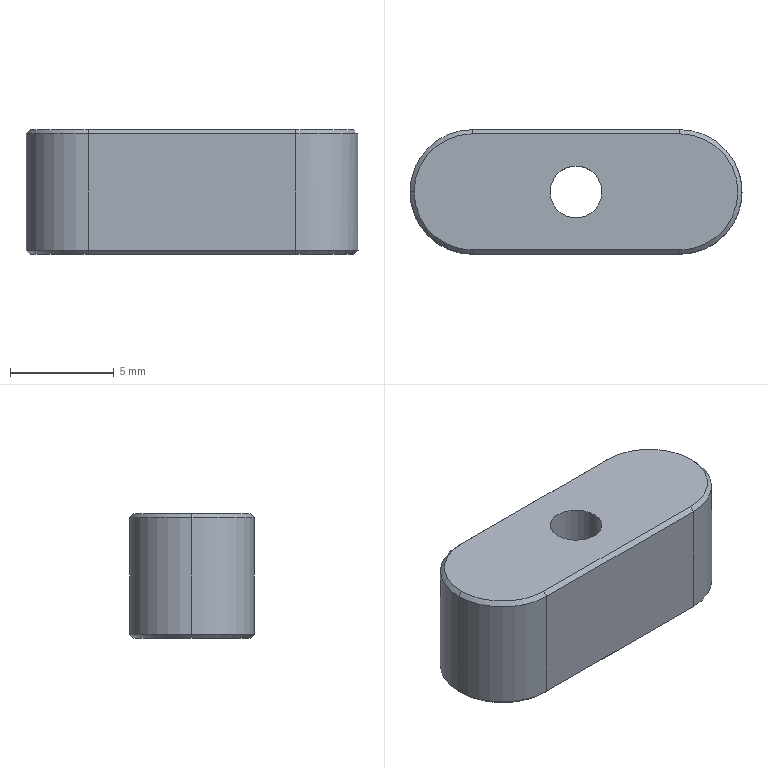Part | NX | features BREP 1 | 1 solid | 19 faces | box 16 x 6 x 6 mm | volume 498.656 mm3 | plane 8 | cone 6 | cylinder 5 | commonest cylinder face diameters 6 x3 2.5 x2
STEP:
#1=CARTESIAN_POINT('',(1.25,0.,-3.));
#2=VERTEX_POINT('',#1);
#3=CARTESIAN_POINT('',(-1.25,0.,-3.));
#4=VERTEX_POINT('',#3);
#5=CARTESIAN_POINT('',(0.,0.,-3.));
#6=DIRECTION('',(0.,0.,-1.));
#7=DIRECTION('',(-1.,0.,0.));
#8=AXIS2_PLACEMENT_3D('',#5,#6,#7);
#9=CIRCLE('',#8,1.25);
#10=EDGE_CURVE('',#2,#4,#9,.T.);
#11=ORIENTED_EDGE('',*,*,#10,.T.);
#12=CARTESIAN_POINT('',(-1.25,0.,3.));
#13=VERTEX_POINT('',#12);
#14=CARTESIAN_POINT('',(-1.25,0.,3.));
#15=DIRECTION('',(0.,0.,1.));
#16=VECTOR('',#15,1000.);
#17=LINE('',#14,#16);
#18=EDGE_CURVE('',#13,#4,#17,.F.);
#19=ORIENTED_EDGE('',*,*,#18,.F.);
#20=CARTESIAN_POINT('',(1.25,0.,3.));
#21=VERTEX_POINT('',#20);
#22=CARTESIAN_POINT('',(0.,0.,3.));
#23=DIRECTION('',(0.,0.,1.));
#24=DIRECTION('',(1.,0.,0.));
#25=AXIS2_PLACEMENT_3D('',#22,#23,#24);
#26=CIRCLE('',#25,1.25);
#27=EDGE_CURVE('',#13,#21,#26,.T.);
#28=ORIENTED_EDGE('',*,*,#27,.T.);
#29=CARTESIAN_POINT('',(1.25,0.,3.));
#30=DIRECTION('',(0.,0.,1.));
#31=VECTOR('',#30,1000.);
#32=LINE('',#29,#31);
#33=EDGE_CURVE('',#21,#2,#32,.F.);
#34=ORIENTED_EDGE('',*,*,#33,.T.);
#35=EDGE_LOOP('',(#11,#19,#28,#34));
#36=FACE_BOUND('',#35,.T.);
#37=CARTESIAN_POINT('',(0.,0.,3.));
#38=DIRECTION('',(0.,0.,1.));
#39=DIRECTION('',(1.,0.,0.));
#40=AXIS2_PLACEMENT_3D('',#37,#38,#39);
#41=CYLINDRICAL_SURFACE('',#40,1.25);
#42=ADVANCED_FACE('',(#36),#41,.F.);
#43=CARTESIAN_POINT('',(-7.8,0.,3.));
#44=VERTEX_POINT('',#43);
#45=CARTESIAN_POINT('',(-5.,-2.8,3.));
#46=VERTEX_POINT('',#45);
#47=CARTESIAN_POINT('',(-5.,0.,3.));
#48=DIRECTION('',(0.,0.,1.));
#49=DIRECTION('',(-1.,0.,0.));
#50=AXIS2_PLACEMENT_3D('',#47,#48,#49);
#51=CIRCLE('',#50,2.8);
#52=EDGE_CURVE('',#44,#46,#51,.T.);
#53=ORIENTED_EDGE('',*,*,#52,.F.);
#54=CARTESIAN_POINT('',(-8.,0.,2.8));
#55=VERTEX_POINT('',#54);
#56=CARTESIAN_POINT('',(-7.8,0.,3.));
#57=DIRECTION('',(-0.7071,0.,-0.7071));
#58=VECTOR('',#57,1000.);
#59=LINE('',#56,#58);
#60=EDGE_CURVE('',#44,#55,#59,.T.);
#61=ORIENTED_EDGE('',*,*,#60,.T.);
#62=CARTESIAN_POINT('',(-5.,-3.,2.8));
#63=VERTEX_POINT('',#62);
#64=CARTESIAN_POINT('',(-5.,0.,2.8));
#65=DIRECTION('',(0.,0.,-1.));
#66=DIRECTION('',(-1.,0.,0.));
#67=AXIS2_PLACEMENT_3D('',#64,#65,#66);
#68=CIRCLE('',#67,3.);
#69=EDGE_CURVE('',#63,#55,#68,.T.);
#70=ORIENTED_EDGE('',*,*,#69,.F.);
#71=CARTESIAN_POINT('',(-5.,-2.8,3.));
#72=DIRECTION('',(0.,-0.7071,-0.7071));
#73=VECTOR('',#72,1000.);
#74=LINE('',#71,#73);
#75=EDGE_CURVE('',#46,#63,#74,.T.);
#76=ORIENTED_EDGE('',*,*,#75,.F.);
#77=EDGE_LOOP('',(#53,#61,#70,#76));
#78=FACE_BOUND('',#77,.T.);
#79=CARTESIAN_POINT('',(-5.,0.,3.));
#80=DIRECTION('',(0.,0.,-1.));
#81=DIRECTION('',(-1.,0.,0.));
#82=AXIS2_PLACEMENT_3D('',#79,#80,#81);
#83=CONICAL_SURFACE('',#82,2.8,0.7854);
#84=ADVANCED_FACE('',(#78),#83,.T.);
#85=CARTESIAN_POINT('',(7.8,0.,-3.));
#86=VERTEX_POINT('',#85);
#87=CARTESIAN_POINT('',(5.,-2.8,-3.));
#88=VERTEX_POINT('',#87);
#89=CARTESIAN_POINT('',(5.,0.,-3.));
#90=DIRECTION('',(0.,0.,-1.));
#91=DIRECTION('',(-1.,0.,0.));
#92=AXIS2_PLACEMENT_3D('',#89,#90,#91);
#93=CIRCLE('',#92,2.8);
#94=EDGE_CURVE('',#86,#88,#93,.T.);
#95=ORIENTED_EDGE('',*,*,#94,.F.);
#96=CARTESIAN_POINT('',(8.,0.,-2.8));
#97=VERTEX_POINT('',#96);
#98=CARTESIAN_POINT('',(8.,0.,-2.8));
#99=DIRECTION('',(0.7071,0.,0.7071));
#100=VECTOR('',#99,1000.);
#101=LINE('',#98,#100);
#102=EDGE_CURVE('',#86,#97,#101,.T.);
#103=ORIENTED_EDGE('',*,*,#102,.T.);
#104=CARTESIAN_POINT('',(5.,-3.,-2.8));
#105=VERTEX_POINT('',#104);
#106=CARTESIAN_POINT('',(5.,0.,-2.8));
#107=DIRECTION('',(0.,0.,1.));
#108=DIRECTION('',(-1.,0.,0.));
#109=AXIS2_PLACEMENT_3D('',#106,#107,#108);
#110=CIRCLE('',#109,3.);
#111=EDGE_CURVE('',#105,#97,#110,.T.);
#112=ORIENTED_EDGE('',*,*,#111,.F.);
#113=CARTESIAN_POINT('',(5.,-3.,-2.8));
#114=DIRECTION('',(0.,0.7071,-0.7071));
#115=VECTOR('',#114,1000.);
#116=LINE('',#113,#115);
#117=EDGE_CURVE('',#105,#88,#116,.T.);
#118=ORIENTED_EDGE('',*,*,#117,.T.);
#119=EDGE_LOOP('',(#95,#103,#112,#118));
#120=FACE_BOUND('',#119,.T.);
#121=CARTESIAN_POINT('',(5.,0.,-2.8));
#122=DIRECTION('',(0.,0.,1.));
#123=DIRECTION('',(1.,0.,0.));
#124=AXIS2_PLACEMENT_3D('',#121,#122,#123);
#125=CONICAL_SURFACE('',#124,3.,0.7854);
#126=ADVANCED_FACE('',(#120),#125,.T.);
#127=ORIENTED_EDGE('',*,*,#69,.T.);
#128=CARTESIAN_POINT('',(-8.,0.,-2.8));
#129=VERTEX_POINT('',#128);
#130=CARTESIAN_POINT('',(-8.,0.,3.));
#131=DIRECTION('',(0.,0.,-1.));
#132=VECTOR('',#131,1000.);
#133=LINE('',#130,#132);
#134=EDGE_CURVE('',#55,#129,#133,.T.);
#135=ORIENTED_EDGE('',*,*,#134,.T.);
#136=CARTESIAN_POINT('',(-5.,-3.,-2.8));
#137=VERTEX_POINT('',#136);
#138=CARTESIAN_POINT('',(-5.,0.,-2.8));
#139=DIRECTION('',(0.,0.,1.));
#140=DIRECTION('',(-1.,0.,0.));
#141=AXIS2_PLACEMENT_3D('',#138,#139,#140);
#142=CIRCLE('',#141,3.);
#143=EDGE_CURVE('',#129,#137,#142,.T.);
#144=ORIENTED_EDGE('',*,*,#143,.T.);
#145=CARTESIAN_POINT('',(-5.,-3.,3.));
#146=DIRECTION('',(0.,0.,-1.));
#147=VECTOR('',#146,1000.);
#148=LINE('',#145,#147);
#149=EDGE_CURVE('',#63,#137,#148,.T.);
#150=ORIENTED_EDGE('',*,*,#149,.F.);
#151=EDGE_LOOP('',(#127,#135,#144,#150));
#152=FACE_BOUND('',#151,.T.);
#153=CARTESIAN_POINT('',(-5.,0.,3.));
#154=DIRECTION('',(0.,0.,-1.));
#155=DIRECTION('',(-1.,0.,0.));
#156=AXIS2_PLACEMENT_3D('',#153,#154,#155);
#157=CYLINDRICAL_SURFACE('',#156,3.);
#158=ADVANCED_FACE('',(#152),#157,.T.);
#159=CARTESIAN_POINT('',(5.,-3.,2.8));
#160=VERTEX_POINT('',#159);
#161=CARTESIAN_POINT('',(5.,-3.,3.));
#162=DIRECTION('',(0.,0.,-1.));
#163=VECTOR('',#162,1000.);
#164=LINE('',#161,#163);
#165=EDGE_CURVE('',#160,#105,#164,.T.);
#166=ORIENTED_EDGE('',*,*,#165,.T.);
#167=ORIENTED_EDGE('',*,*,#111,.T.);
#168=CARTESIAN_POINT('',(5.,3.,-2.8));
#169=VERTEX_POINT('',#168);
#170=CARTESIAN_POINT('',(5.,0.,-2.8));
#171=DIRECTION('',(0.,0.,1.));
#172=DIRECTION('',(-1.,0.,0.));
#173=AXIS2_PLACEMENT_3D('',#170,#171,#172);
#174=CIRCLE('',#173,3.);
#175=EDGE_CURVE('',#97,#169,#174,.T.);
#176=ORIENTED_EDGE('',*,*,#175,.T.);
#177=CARTESIAN_POINT('',(5.,3.,2.8));
#178=VERTEX_POINT('',#177);
#179=CARTESIAN_POINT('',(5.,3.,3.));
#180=DIRECTION('',(0.,0.,-1.));
#181=VECTOR('',#180,1000.);
#182=LINE('',#179,#181);
#183=EDGE_CURVE('',#178,#169,#182,.T.);
#184=ORIENTED_EDGE('',*,*,#183,.F.);
#185=CARTESIAN_POINT('',(5.,0.,2.8));
#186=DIRECTION('',(0.,0.,-1.));
#187=DIRECTION('',(-1.,0.,0.));
#188=AXIS2_PLACEMENT_3D('',#185,#186,#187);
#189=CIRCLE('',#188,3.);
#190=EDGE_CURVE('',#178,#160,#189,.T.);
#191=ORIENTED_EDGE('',*,*,#190,.T.);
#192=EDGE_LOOP('',(#166,#167,#176,#184,#191));
#193=FACE_BOUND('',#192,.T.);
#194=CARTESIAN_POINT('',(5.,0.,3.));
#195=DIRECTION('',(0.,0.,-1.));
#196=DIRECTION('',(-1.,0.,0.));
#197=AXIS2_PLACEMENT_3D('',#194,#195,#196);
#198=CYLINDRICAL_SURFACE('',#197,3.);
#199=ADVANCED_FACE('',(#193),#198,.T.);
#200=ORIENTED_EDGE('',*,*,#183,.T.);
#201=CARTESIAN_POINT('',(-5.,3.,-2.8));
#202=VERTEX_POINT('',#201);
#203=CARTESIAN_POINT('',(-5.,3.,-2.8));
#204=DIRECTION('',(-1.,0.,0.));
#205=VECTOR('',#204,1000.);
#206=LINE('',#203,#205);
#207=EDGE_CURVE('',#169,#202,#206,.T.);
#208=ORIENTED_EDGE('',*,*,#207,.T.);
#209=CARTESIAN_POINT('',(-5.,3.,2.8));
#210=VERTEX_POINT('',#209);
#211=CARTESIAN_POINT('',(-5.,3.,3.));
#212=DIRECTION('',(0.,0.,-1.));
#213=VECTOR('',#212,1000.);
#214=LINE('',#211,#213);
#215=EDGE_CURVE('',#210,#202,#214,.T.);
#216=ORIENTED_EDGE('',*,*,#215,.F.);
#217=CARTESIAN_POINT('',(-5.,3.,2.8));
#218=DIRECTION('',(1.,0.,0.));
#219=VECTOR('',#218,1000.);
#220=LINE('',#217,#219);
#221=EDGE_CURVE('',#210,#178,#220,.T.);
#222=ORIENTED_EDGE('',*,*,#221,.T.);
#223=EDGE_LOOP('',(#200,#208,#216,#222));
#224=FACE_BOUND('',#223,.T.);
#225=CARTESIAN_POINT('',(-5.,3.,3.));
#226=DIRECTION('',(0.,-1.,0.));
#227=DIRECTION('',(-1.,0.,0.));
#228=AXIS2_PLACEMENT_3D('',#225,#226,#227);
#229=PLANE('',#228);
#230=ADVANCED_FACE('',(#224),#229,.F.);
#231=ORIENTED_EDGE('',*,*,#134,.F.);
#232=CARTESIAN_POINT('',(-5.,0.,2.8));
#233=DIRECTION('',(0.,0.,-1.));
#234=DIRECTION('',(-1.,0.,0.));
#235=AXIS2_PLACEMENT_3D('',#232,#233,#234);
#236=CIRCLE('',#235,3.);
#237=EDGE_CURVE('',#55,#210,#236,.T.);
#238=ORIENTED_EDGE('',*,*,#237,.T.);
#239=ORIENTED_EDGE('',*,*,#215,.T.);
#240=CARTESIAN_POINT('',(-5.,0.,-2.8));
#241=DIRECTION('',(0.,0.,1.));
#242=DIRECTION('',(-1.,0.,0.));
#243=AXIS2_PLACEMENT_3D('',#240,#241,#242);
#244=CIRCLE('',#243,3.);
#245=EDGE_CURVE('',#202,#129,#244,.T.);
#246=ORIENTED_EDGE('',*,*,#245,.T.);
#247=EDGE_LOOP('',(#231,#238,#239,#246));
#248=FACE_BOUND('',#247,.T.);
#249=CARTESIAN_POINT('',(-5.,0.,3.));
#250=DIRECTION('',(0.,0.,-1.));
#251=DIRECTION('',(-1.,0.,0.));
#252=AXIS2_PLACEMENT_3D('',#249,#250,#251);
#253=CYLINDRICAL_SURFACE('',#252,3.);
#254=ADVANCED_FACE('',(#248),#253,.T.);
#255=ORIENTED_EDGE('',*,*,#149,.T.);
#256=CARTESIAN_POINT('',(5.,-3.,-2.8));
#257=DIRECTION('',(1.,0.,0.));
#258=VECTOR('',#257,1000.);
#259=LINE('',#256,#258);
#260=EDGE_CURVE('',#137,#105,#259,.T.);
#261=ORIENTED_EDGE('',*,*,#260,.T.);
#262=ORIENTED_EDGE('',*,*,#165,.F.);
#263=CARTESIAN_POINT('',(-5.,-3.,2.8));
#264=DIRECTION('',(-1.,0.,0.));
#265=VECTOR('',#264,1000.);
#266=LINE('',#263,#265);
#267=EDGE_CURVE('',#160,#63,#266,.T.);
#268=ORIENTED_EDGE('',*,*,#267,.T.);
#269=EDGE_LOOP('',(#255,#261,#262,#268));
#270=FACE_BOUND('',#269,.T.);
#271=CARTESIAN_POINT('',(-5.,-3.,3.));
#272=DIRECTION('',(0.,1.,0.));
#273=DIRECTION('',(1.,0.,0.));
#274=AXIS2_PLACEMENT_3D('',#271,#272,#273);
#275=PLANE('',#274);
#276=ADVANCED_FACE('',(#270),#275,.F.);
#277=CARTESIAN_POINT('',(5.,-2.8,3.));
#278=VERTEX_POINT('',#277);
#279=CARTESIAN_POINT('',(5.,-2.8,3.));
#280=DIRECTION('',(1.,0.,0.));
#281=VECTOR('',#280,1000.);
#282=LINE('',#279,#281);
#283=EDGE_CURVE('',#46,#278,#282,.T.);
#284=ORIENTED_EDGE('',*,*,#283,.T.);
#285=CARTESIAN_POINT('',(5.,2.8,3.));
#286=VERTEX_POINT('',#285);
#287=CARTESIAN_POINT('',(5.,0.,3.));
#288=DIRECTION('',(0.,0.,1.));
#289=DIRECTION('',(-1.,0.,0.));
#290=AXIS2_PLACEMENT_3D('',#287,#288,#289);
#291=CIRCLE('',#290,2.8);
#292=EDGE_CURVE('',#278,#286,#291,.T.);
#293=ORIENTED_EDGE('',*,*,#292,.T.);
#294=CARTESIAN_POINT('',(-5.,2.8,3.));
#295=VERTEX_POINT('',#294);
#296=CARTESIAN_POINT('',(5.,2.8,3.));
#297=DIRECTION('',(-1.,0.,0.));
#298=VECTOR('',#297,1000.);
#299=LINE('',#296,#298);
#300=EDGE_CURVE('',#286,#295,#299,.T.);
#301=ORIENTED_EDGE('',*,*,#300,.T.);
#302=CARTESIAN_POINT('',(-5.,0.,3.));
#303=DIRECTION('',(0.,0.,1.));
#304=DIRECTION('',(-1.,0.,0.));
#305=AXIS2_PLACEMENT_3D('',#302,#303,#304);
#306=CIRCLE('',#305,2.8);
#307=EDGE_CURVE('',#295,#44,#306,.T.);
#308=ORIENTED_EDGE('',*,*,#307,.T.);
#309=ORIENTED_EDGE('',*,*,#52,.T.);
#310=EDGE_LOOP('',(#284,#293,#301,#308,#309));
#311=FACE_BOUND('',#310,.T.);
#312=CARTESIAN_POINT('',(0.,0.,3.));
#313=DIRECTION('',(0.,0.,1.));
#314=DIRECTION('',(1.,0.,0.));
#315=AXIS2_PLACEMENT_3D('',#312,#313,#314);
#316=CIRCLE('',#315,1.25);
#317=EDGE_CURVE('',#21,#13,#316,.T.);
#318=ORIENTED_EDGE('',*,*,#317,.F.);
#319=ORIENTED_EDGE('',*,*,#27,.F.);
#320=EDGE_LOOP('',(#318,#319));
#321=FACE_BOUND('',#320,.T.);
#322=CARTESIAN_POINT('',(5.,0.,3.));
#323=DIRECTION('',(0.,0.,-1.));
#324=DIRECTION('',(0.,-1.,0.));
#325=AXIS2_PLACEMENT_3D('',#322,#323,#324);
#326=PLANE('',#325);
#327=ADVANCED_FACE('',(#311,#321),#326,.F.);
#328=CARTESIAN_POINT('',(-5.,-2.8,-3.));
#329=VERTEX_POINT('',#328);
#330=CARTESIAN_POINT('',(-5.,2.8,-3.));
#331=VERTEX_POINT('',#330);
#332=CARTESIAN_POINT('',(-5.,0.,-3.));
#333=DIRECTION('',(0.,0.,-1.));
#334=DIRECTION('',(-1.,0.,0.));
#335=AXIS2_PLACEMENT_3D('',#332,#333,#334);
#336=CIRCLE('',#335,2.8);
#337=EDGE_CURVE('',#329,#331,#336,.T.);
#338=ORIENTED_EDGE('',*,*,#337,.T.);
#339=CARTESIAN_POINT('',(5.,2.8,-3.));
#340=VERTEX_POINT('',#339);
#341=CARTESIAN_POINT('',(5.,2.8,-3.));
#342=DIRECTION('',(1.,0.,0.));
#343=VECTOR('',#342,1000.);
#344=LINE('',#341,#343);
#345=EDGE_CURVE('',#331,#340,#344,.T.);
#346=ORIENTED_EDGE('',*,*,#345,.T.);
#347=CARTESIAN_POINT('',(5.,0.,-3.));
#348=DIRECTION('',(0.,0.,-1.));
#349=DIRECTION('',(-1.,0.,0.));
#350=AXIS2_PLACEMENT_3D('',#347,#348,#349);
#351=CIRCLE('',#350,2.8);
#352=EDGE_CURVE('',#340,#86,#351,.T.);
#353=ORIENTED_EDGE('',*,*,#352,.T.);
#354=ORIENTED_EDGE('',*,*,#94,.T.);
#355=CARTESIAN_POINT('',(-5.,-2.8,-3.));
#356=DIRECTION('',(-1.,0.,0.));
#357=VECTOR('',#356,1000.);
#358=LINE('',#355,#357);
#359=EDGE_CURVE('',#88,#329,#358,.T.);
#360=ORIENTED_EDGE('',*,*,#359,.T.);
#361=EDGE_LOOP('',(#338,#346,#353,#354,#360));
#362=FACE_BOUND('',#361,.T.);
#363=ORIENTED_EDGE('',*,*,#10,.F.);
#364=CARTESIAN_POINT('',(0.,0.,-3.));
#365=DIRECTION('',(0.,0.,-1.));
#366=DIRECTION('',(-1.,0.,0.));
#367=AXIS2_PLACEMENT_3D('',#364,#365,#366);
#368=CIRCLE('',#367,1.25);
#369=EDGE_CURVE('',#4,#2,#368,.T.);
#370=ORIENTED_EDGE('',*,*,#369,.F.);
#371=EDGE_LOOP('',(#363,#370));
#372=FACE_BOUND('',#371,.T.);
#373=CARTESIAN_POINT('',(5.,0.,-3.));
#374=DIRECTION('',(0.,0.,-1.));
#375=DIRECTION('',(0.,-1.,0.));
#376=AXIS2_PLACEMENT_3D('',#373,#374,#375);
#377=PLANE('',#376);
#378=ADVANCED_FACE('',(#362,#372),#377,.T.);
#379=CARTESIAN_POINT('',(-5.,-2.8,-3.));
#380=DIRECTION('',(0.,-0.7071,0.7071));
#381=VECTOR('',#380,1000.);
#382=LINE('',#379,#381);
#383=EDGE_CURVE('',#329,#137,#382,.T.);
#384=ORIENTED_EDGE('',*,*,#383,.F.);
#385=ORIENTED_EDGE('',*,*,#359,.F.);
#386=ORIENTED_EDGE('',*,*,#117,.F.);
#387=ORIENTED_EDGE('',*,*,#260,.F.);
#388=EDGE_LOOP('',(#384,#385,#386,#387));
#389=FACE_BOUND('',#388,.T.);
#390=CARTESIAN_POINT('',(-5.,-3.,-2.8));
#391=DIRECTION('',(0.,-0.7071,-0.7071));
#392=DIRECTION('',(0.,-0.7071,0.7071));
#393=AXIS2_PLACEMENT_3D('',#390,#391,#392);
#394=PLANE('',#393);
#395=ADVANCED_FACE('',(#389),#394,.T.);
#396=ORIENTED_EDGE('',*,*,#102,.F.);
#397=ORIENTED_EDGE('',*,*,#352,.F.);
#398=CARTESIAN_POINT('',(5.,3.,-2.8));
#399=DIRECTION('',(0.,-0.7071,-0.7071));
#400=VECTOR('',#399,1000.);
#401=LINE('',#398,#400);
#402=EDGE_CURVE('',#169,#340,#401,.T.);
#403=ORIENTED_EDGE('',*,*,#402,.F.);
#404=ORIENTED_EDGE('',*,*,#175,.F.);
#405=EDGE_LOOP('',(#396,#397,#403,#404));
#406=FACE_BOUND('',#405,.T.);
#407=CARTESIAN_POINT('',(5.,0.,-2.8));
#408=DIRECTION('',(0.,0.,1.));
#409=DIRECTION('',(1.,0.,0.));
#410=AXIS2_PLACEMENT_3D('',#407,#408,#409);
#411=CONICAL_SURFACE('',#410,3.,0.7854);
#412=ADVANCED_FACE('',(#406),#411,.T.);
#413=ORIENTED_EDGE('',*,*,#383,.T.);
#414=ORIENTED_EDGE('',*,*,#143,.F.);
#415=ORIENTED_EDGE('',*,*,#245,.F.);
#416=CARTESIAN_POINT('',(-5.,2.8,-3.));
#417=DIRECTION('',(0.,0.7071,0.7071));
#418=VECTOR('',#417,1000.);
#419=LINE('',#416,#418);
#420=EDGE_CURVE('',#331,#202,#419,.T.);
#421=ORIENTED_EDGE('',*,*,#420,.F.);
#422=ORIENTED_EDGE('',*,*,#337,.F.);
#423=EDGE_LOOP('',(#413,#414,#415,#421,#422));
#424=FACE_BOUND('',#423,.T.);
#425=CARTESIAN_POINT('',(-5.,0.,-2.8));
#426=DIRECTION('',(0.,0.,1.));
#427=DIRECTION('',(1.,0.,0.));
#428=AXIS2_PLACEMENT_3D('',#425,#426,#427);
#429=CONICAL_SURFACE('',#428,3.,0.7854);
#430=ADVANCED_FACE('',(#424),#429,.T.);
#431=ORIENTED_EDGE('',*,*,#402,.T.);
#432=ORIENTED_EDGE('',*,*,#345,.F.);
#433=ORIENTED_EDGE('',*,*,#420,.T.);
#434=ORIENTED_EDGE('',*,*,#207,.F.);
#435=EDGE_LOOP('',(#431,#432,#433,#434));
#436=FACE_BOUND('',#435,.T.);
#437=CARTESIAN_POINT('',(-5.,3.,-2.8));
#438=DIRECTION('',(0.,0.7071,-0.7071));
#439=DIRECTION('',(-1.,0.,0.));
#440=AXIS2_PLACEMENT_3D('',#437,#438,#439);
#441=PLANE('',#440);
#442=ADVANCED_FACE('',(#436),#441,.T.);
#443=ORIENTED_EDGE('',*,*,#60,.F.);
#444=ORIENTED_EDGE('',*,*,#307,.F.);
#445=CARTESIAN_POINT('',(-5.,3.,2.8));
#446=DIRECTION('',(0.,-0.7071,0.7071));
#447=VECTOR('',#446,1000.);
#448=LINE('',#445,#447);
#449=EDGE_CURVE('',#210,#295,#448,.T.);
#450=ORIENTED_EDGE('',*,*,#449,.F.);
#451=ORIENTED_EDGE('',*,*,#237,.F.);
#452=EDGE_LOOP('',(#443,#444,#450,#451));
#453=FACE_BOUND('',#452,.T.);
#454=CARTESIAN_POINT('',(-5.,0.,3.));
#455=DIRECTION('',(0.,0.,-1.));
#456=DIRECTION('',(-1.,0.,0.));
#457=AXIS2_PLACEMENT_3D('',#454,#455,#456);
#458=CONICAL_SURFACE('',#457,2.8,0.7854);
#459=ADVANCED_FACE('',(#453),#458,.T.);
#460=ORIENTED_EDGE('',*,*,#75,.T.);
#461=ORIENTED_EDGE('',*,*,#267,.F.);
#462=CARTESIAN_POINT('',(5.,-2.8,3.));
#463=DIRECTION('',(0.,-0.7071,-0.7071));
#464=VECTOR('',#463,1000.);
#465=LINE('',#462,#464);
#466=EDGE_CURVE('',#278,#160,#465,.T.);
#467=ORIENTED_EDGE('',*,*,#466,.F.);
#468=ORIENTED_EDGE('',*,*,#283,.F.);
#469=EDGE_LOOP('',(#460,#461,#467,#468));
#470=FACE_BOUND('',#469,.T.);
#471=CARTESIAN_POINT('',(5.,-2.8,3.));
#472=DIRECTION('',(0.,0.7071,-0.7071));
#473=DIRECTION('',(-1.,0.,0.));
#474=AXIS2_PLACEMENT_3D('',#471,#472,#473);
#475=PLANE('',#474);
#476=ADVANCED_FACE('',(#470),#475,.F.);
#477=ORIENTED_EDGE('',*,*,#449,.T.);
#478=ORIENTED_EDGE('',*,*,#300,.F.);
#479=CARTESIAN_POINT('',(5.,3.,2.8));
#480=DIRECTION('',(0.,-0.7071,0.7071));
#481=VECTOR('',#480,1000.);
#482=LINE('',#479,#481);
#483=EDGE_CURVE('',#178,#286,#482,.T.);
#484=ORIENTED_EDGE('',*,*,#483,.F.);
#485=ORIENTED_EDGE('',*,*,#221,.F.);
#486=EDGE_LOOP('',(#477,#478,#484,#485));
#487=FACE_BOUND('',#486,.T.);
#488=CARTESIAN_POINT('',(5.,2.8,3.));
#489=DIRECTION('',(0.,-0.7071,-0.7071));
#490=DIRECTION('',(0.,0.7071,-0.7071));
#491=AXIS2_PLACEMENT_3D('',#488,#489,#490);
#492=PLANE('',#491);
#493=ADVANCED_FACE('',(#487),#492,.F.);
#494=ORIENTED_EDGE('',*,*,#466,.T.);
#495=ORIENTED_EDGE('',*,*,#190,.F.);
#496=ORIENTED_EDGE('',*,*,#483,.T.);
#497=ORIENTED_EDGE('',*,*,#292,.F.);
#498=EDGE_LOOP('',(#494,#495,#496,#497));
#499=FACE_BOUND('',#498,.T.);
#500=CARTESIAN_POINT('',(5.,0.,3.));
#501=DIRECTION('',(0.,0.,-1.));
#502=DIRECTION('',(-1.,0.,0.));
#503=AXIS2_PLACEMENT_3D('',#500,#501,#502);
#504=CONICAL_SURFACE('',#503,2.8,0.7854);
#505=ADVANCED_FACE('',(#499),#504,.T.);
#506=ORIENTED_EDGE('',*,*,#18,.T.);
#507=ORIENTED_EDGE('',*,*,#369,.T.);
#508=ORIENTED_EDGE('',*,*,#33,.F.);
#509=ORIENTED_EDGE('',*,*,#317,.T.);
#510=EDGE_LOOP('',(#506,#507,#508,#509));
#511=FACE_BOUND('',#510,.T.);
#512=CARTESIAN_POINT('',(0.,0.,3.));
#513=DIRECTION('',(0.,0.,1.));
#514=DIRECTION('',(1.,0.,0.));
#515=AXIS2_PLACEMENT_3D('',#512,#513,#514);
#516=CYLINDRICAL_SURFACE('',#515,1.25);
#517=ADVANCED_FACE('',(#511),#516,.F.);
#518=CLOSED_SHELL('',(#42,#84,#126,#158,#199,#230,#254,#276,#327,#378,#395,#412,#430,#442,#459,#476,#493,#505,#517));
#519=MANIFOLD_SOLID_BREP('',#518);
#520=(LENGTH_UNIT()NAMED_UNIT(*)SI_UNIT(.MILLI.,.METRE.));
#521=UNCERTAINTY_MEASURE_WITH_UNIT(LENGTH_MEASURE(0.00001),#520,'','');
#522=(NAMED_UNIT(*)PLANE_ANGLE_UNIT()SI_UNIT($,.RADIAN.));
#523=(NAMED_UNIT(*)SI_UNIT($,.STERADIAN.)SOLID_ANGLE_UNIT());
#524=(GEOMETRIC_REPRESENTATION_CONTEXT(3)GLOBAL_UNCERTAINTY_ASSIGNED_CONTEXT((#521))GLOBAL_UNIT_ASSIGNED_CONTEXT((#520,#522,#523))REPRESENTATION_CONTEXT('',''));
#525=ADVANCED_BREP_SHAPE_REPRESENTATION('',(#519),#524);